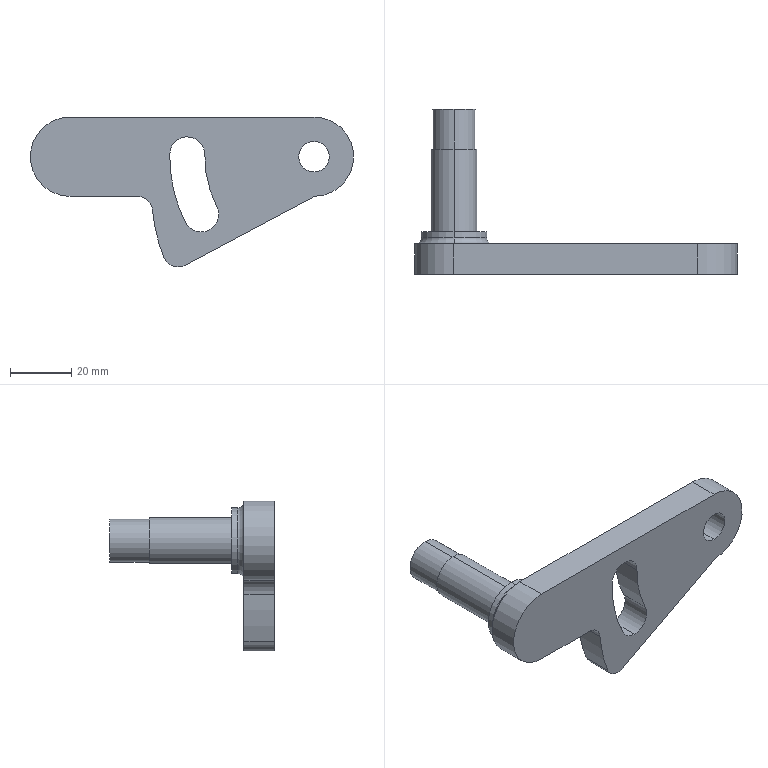Part | SolidWorks | features ICE 3, Fillet 2, Extrusion 1 | 1 solid | 30 faces | box 105.906 x 54 x 49.114 mm | volume 37118 mm3 | cylinder 20 | plane 8 | torus 2 | commonest cylinder face diameters 10 x5 11.5 x3 14 x2 15 x2 21.5 x2 26.001 x2
STEP:
#1=CARTESIAN_POINT('',(0.09446,54.,-6.));
#2=VERTEX_POINT('',#1);
#3=CARTESIAN_POINT('',(0.09446,54.,-20.));
#4=VERTEX_POINT('',#3);
#5=CARTESIAN_POINT('',(0.09446,54.,-13.));
#6=DIRECTION('',(0.,1.,0.));
#7=DIRECTION('',(0.,0.,1.));
#8=AXIS2_PLACEMENT_3D('',#5,#6,#7);
#9=CIRCLE('',#8,7.);
#10=EDGE_CURVE('',#2,#4,#9,.T.);
#11=ORIENTED_EDGE('',*,*,#10,.F.);
#12=CARTESIAN_POINT('',(0.09446,41.,-6.));
#13=VERTEX_POINT('',#12);
#14=CARTESIAN_POINT('',(0.09446,54.,-6.));
#15=DIRECTION('',(0.,-1.,0.));
#16=VECTOR('',#15,1000.);
#17=LINE('',#14,#16);
#18=EDGE_CURVE('',#2,#13,#17,.T.);
#19=ORIENTED_EDGE('',*,*,#18,.T.);
#20=CARTESIAN_POINT('',(0.09446,41.,-20.));
#21=VERTEX_POINT('',#20);
#22=CARTESIAN_POINT('',(0.09446,41.,-13.));
#23=DIRECTION('',(0.,1.,0.));
#24=DIRECTION('',(0.,0.,1.));
#25=AXIS2_PLACEMENT_3D('',#22,#23,#24);
#26=CIRCLE('',#25,7.);
#27=EDGE_CURVE('',#13,#21,#26,.T.);
#28=ORIENTED_EDGE('',*,*,#27,.T.);
#29=CARTESIAN_POINT('',(0.09446,54.,-20.));
#30=DIRECTION('',(0.,-1.,0.));
#31=VECTOR('',#30,1000.);
#32=LINE('',#29,#31);
#33=EDGE_CURVE('',#4,#21,#32,.T.);
#34=ORIENTED_EDGE('',*,*,#33,.F.);
#35=EDGE_LOOP('',(#11,#19,#28,#34));
#36=FACE_OUTER_BOUND('',#35,.T.);
#37=CARTESIAN_POINT('',(0.09446,54.,-13.));
#38=DIRECTION('',(0.,-1.,0.));
#39=DIRECTION('',(0.,0.,-1.));
#40=AXIS2_PLACEMENT_3D('',#37,#38,#39);
#41=CYLINDRICAL_SURFACE('',#40,7.);
#42=ADVANCED_FACE('',(#36),#41,.T.);
#43=CARTESIAN_POINT('',(0.09446,41.,-5.5));
#44=VERTEX_POINT('',#43);
#45=CARTESIAN_POINT('',(0.09446,41.,-20.5));
#46=VERTEX_POINT('',#45);
#47=CARTESIAN_POINT('',(0.09446,41.,-13.));
#48=DIRECTION('',(0.,1.,0.));
#49=DIRECTION('',(0.,0.,1.));
#50=AXIS2_PLACEMENT_3D('',#47,#48,#49);
#51=CIRCLE('',#50,7.5);
#52=EDGE_CURVE('',#44,#46,#51,.T.);
#53=ORIENTED_EDGE('',*,*,#52,.F.);
#54=CARTESIAN_POINT('',(0.09446,14.,-5.5));
#55=VERTEX_POINT('',#54);
#56=CARTESIAN_POINT('',(0.09446,41.,-5.5));
#57=DIRECTION('',(0.,-1.,0.));
#58=VECTOR('',#57,1000.);
#59=LINE('',#56,#58);
#60=EDGE_CURVE('',#44,#55,#59,.T.);
#61=ORIENTED_EDGE('',*,*,#60,.T.);
#62=CARTESIAN_POINT('',(0.09446,14.,-20.5));
#63=VERTEX_POINT('',#62);
#64=CARTESIAN_POINT('',(0.09446,14.,-13.));
#65=DIRECTION('',(0.,1.,0.));
#66=DIRECTION('',(0.,0.,1.));
#67=AXIS2_PLACEMENT_3D('',#64,#65,#66);
#68=CIRCLE('',#67,7.5);
#69=EDGE_CURVE('',#55,#63,#68,.T.);
#70=ORIENTED_EDGE('',*,*,#69,.T.);
#71=CARTESIAN_POINT('',(0.09446,41.,-20.5));
#72=DIRECTION('',(0.,-1.,0.));
#73=VECTOR('',#72,1000.);
#74=LINE('',#71,#73);
#75=EDGE_CURVE('',#46,#63,#74,.T.);
#76=ORIENTED_EDGE('',*,*,#75,.F.);
#77=EDGE_LOOP('',(#53,#61,#70,#76));
#78=FACE_OUTER_BOUND('',#77,.T.);
#79=CARTESIAN_POINT('',(0.09446,41.,-13.));
#80=DIRECTION('',(0.,-1.,0.));
#81=DIRECTION('',(0.,0.,-1.));
#82=AXIS2_PLACEMENT_3D('',#79,#80,#81);
#83=CYLINDRICAL_SURFACE('',#82,7.5);
#84=ADVANCED_FACE('',(#78),#83,.T.);
#85=CARTESIAN_POINT('',(0.09446,12.,-23.75));
#86=VERTEX_POINT('',#85);
#87=CARTESIAN_POINT('',(0.09446,12.,-2.25));
#88=VERTEX_POINT('',#87);
#89=CARTESIAN_POINT('',(0.09446,12.,-13.));
#90=DIRECTION('',(0.,1.,0.));
#91=DIRECTION('',(0.,0.,1.));
#92=AXIS2_PLACEMENT_3D('',#89,#90,#91);
#93=CIRCLE('',#92,10.75);
#94=EDGE_CURVE('',#86,#88,#93,.T.);
#95=ORIENTED_EDGE('',*,*,#94,.F.);
#96=CARTESIAN_POINT('',(0.09446,10.,-25.75));
#97=VERTEX_POINT('',#96);
#98=CARTESIAN_POINT('',(0.09446,12.,-25.75));
#99=DIRECTION('',(1.,0.,0.));
#100=DIRECTION('',(0.,0.,-1.));
#101=AXIS2_PLACEMENT_3D('',#98,#99,#100);
#102=CIRCLE('',#101,2.);
#103=EDGE_CURVE('',#86,#97,#102,.T.);
#104=ORIENTED_EDGE('',*,*,#103,.T.);
#105=CARTESIAN_POINT('',(0.09446,10.,-0.25));
#106=VERTEX_POINT('',#105);
#107=CARTESIAN_POINT('',(0.09446,10.,-13.));
#108=DIRECTION('',(0.,-1.,0.));
#109=DIRECTION('',(0.,0.,1.));
#110=AXIS2_PLACEMENT_3D('',#107,#108,#109);
#111=CIRCLE('',#110,12.75);
#112=EDGE_CURVE('',#106,#97,#111,.T.);
#113=ORIENTED_EDGE('',*,*,#112,.F.);
#114=CARTESIAN_POINT('',(0.09446,12.,-0.25));
#115=DIRECTION('',(-1.,0.,0.));
#116=DIRECTION('',(0.,0.,1.));
#117=AXIS2_PLACEMENT_3D('',#114,#115,#116);
#118=CIRCLE('',#117,2.);
#119=EDGE_CURVE('',#88,#106,#118,.T.);
#120=ORIENTED_EDGE('',*,*,#119,.F.);
#121=EDGE_LOOP('',(#95,#104,#113,#120));
#122=FACE_OUTER_BOUND('',#121,.T.);
#123=CARTESIAN_POINT('',(0.09446,12.,-13.));
#124=DIRECTION('',(0.,1.,0.));
#125=DIRECTION('',(0.,0.,1.));
#126=AXIS2_PLACEMENT_3D('',#123,#124,#125);
#127=TOROIDAL_SURFACE('',#126,12.75,2.);
#128=ADVANCED_FACE('',(#122),#127,.F.);
#129=CARTESIAN_POINT('',(0.09446,14.,-2.25));
#130=VERTEX_POINT('',#129);
#131=CARTESIAN_POINT('',(0.09446,14.,-23.75));
#132=VERTEX_POINT('',#131);
#133=CARTESIAN_POINT('',(0.09446,14.,-13.));
#134=DIRECTION('',(0.,1.,0.));
#135=DIRECTION('',(0.,0.,1.));
#136=AXIS2_PLACEMENT_3D('',#133,#134,#135);
#137=CIRCLE('',#136,10.75);
#138=EDGE_CURVE('',#130,#132,#137,.T.);
#139=ORIENTED_EDGE('',*,*,#138,.F.);
#140=CARTESIAN_POINT('',(0.09446,14.,-2.25));
#141=DIRECTION('',(0.,-1.,0.));
#142=VECTOR('',#141,1000.);
#143=LINE('',#140,#142);
#144=EDGE_CURVE('',#130,#88,#143,.T.);
#145=ORIENTED_EDGE('',*,*,#144,.T.);
#146=CARTESIAN_POINT('',(0.09446,12.,-13.));
#147=DIRECTION('',(0.,1.,0.));
#148=DIRECTION('',(0.,0.,1.));
#149=AXIS2_PLACEMENT_3D('',#146,#147,#148);
#150=CIRCLE('',#149,10.75);
#151=EDGE_CURVE('',#88,#86,#150,.T.);
#152=ORIENTED_EDGE('',*,*,#151,.T.);
#153=CARTESIAN_POINT('',(0.09446,14.,-23.75));
#154=DIRECTION('',(0.,-1.,0.));
#155=VECTOR('',#154,1000.);
#156=LINE('',#153,#155);
#157=EDGE_CURVE('',#132,#86,#156,.T.);
#158=ORIENTED_EDGE('',*,*,#157,.F.);
#159=EDGE_LOOP('',(#139,#145,#152,#158));
#160=FACE_OUTER_BOUND('',#159,.T.);
#161=CARTESIAN_POINT('',(0.09446,14.,-13.));
#162=DIRECTION('',(0.,-1.,0.));
#163=DIRECTION('',(0.,0.,-1.));
#164=AXIS2_PLACEMENT_3D('',#161,#162,#163);
#165=CYLINDRICAL_SURFACE('',#164,10.75);
#166=ADVANCED_FACE('',(#160),#165,.T.);
#167=CARTESIAN_POINT('',(35.469,10.,-49.114));
#168=VERTEX_POINT('',#167);
#169=CARTESIAN_POINT('',(30.834,10.,-45.991));
#170=VERTEX_POINT('',#169);
#171=CARTESIAN_POINT('',(35.469,10.,-44.114));
#172=DIRECTION('',(0.,1.,0.));
#173=DIRECTION('',(0.,0.,1.));
#174=AXIS2_PLACEMENT_3D('',#171,#172,#173);
#175=CIRCLE('',#174,5.);
#176=EDGE_CURVE('',#168,#170,#175,.T.);
#177=ORIENTED_EDGE('',*,*,#176,.F.);
#178=CARTESIAN_POINT('',(35.469,0.,-49.114));
#179=VERTEX_POINT('',#178);
#180=CARTESIAN_POINT('',(35.469,10.,-49.114));
#181=DIRECTION('',(0.,-1.,0.));
#182=VECTOR('',#181,1000.);
#183=LINE('',#180,#182);
#184=EDGE_CURVE('',#168,#179,#183,.T.);
#185=ORIENTED_EDGE('',*,*,#184,.T.);
#186=CARTESIAN_POINT('',(30.834,0.,-45.991));
#187=VERTEX_POINT('',#186);
#188=CARTESIAN_POINT('',(35.469,0.,-44.114));
#189=DIRECTION('',(0.,-1.,0.));
#190=DIRECTION('',(0.,0.,1.));
#191=AXIS2_PLACEMENT_3D('',#188,#189,#190);
#192=CIRCLE('',#191,5.);
#193=EDGE_CURVE('',#187,#179,#192,.T.);
#194=ORIENTED_EDGE('',*,*,#193,.F.);
#195=CARTESIAN_POINT('',(30.834,10.,-45.991));
#196=DIRECTION('',(0.,-1.,0.));
#197=VECTOR('',#196,1000.);
#198=LINE('',#195,#197);
#199=EDGE_CURVE('',#170,#187,#198,.T.);
#200=ORIENTED_EDGE('',*,*,#199,.F.);
#201=EDGE_LOOP('',(#177,#185,#194,#200));
#202=FACE_OUTER_BOUND('',#201,.T.);
#203=CARTESIAN_POINT('',(35.469,10.,-44.114));
#204=DIRECTION('',(0.,-1.,0.));
#205=DIRECTION('',(0.,0.,-1.));
#206=AXIS2_PLACEMENT_3D('',#203,#204,#205);
#207=CYLINDRICAL_SURFACE('',#206,5.);
#208=ADVANCED_FACE('',(#202),#207,.T.);
#209=CARTESIAN_POINT('',(48.162,10.,-29.261));
#210=VERTEX_POINT('',#209);
#211=CARTESIAN_POINT('',(43.041,10.,-37.626));
#212=VERTEX_POINT('',#211);
#213=CARTESIAN_POINT('',(43.041,10.,-31.876));
#214=DIRECTION('',(0.,1.,0.));
#215=DIRECTION('',(0.,0.,1.));
#216=AXIS2_PLACEMENT_3D('',#213,#214,#215);
#217=CIRCLE('',#216,5.75);
#218=EDGE_CURVE('',#210,#212,#217,.T.);
#219=ORIENTED_EDGE('',*,*,#218,.T.);
#220=CARTESIAN_POINT('',(43.041,0.,-37.626));
#221=VERTEX_POINT('',#220);
#222=CARTESIAN_POINT('',(43.041,10.,-37.626));
#223=DIRECTION('',(0.,-1.,0.));
#224=VECTOR('',#223,1000.);
#225=LINE('',#222,#224);
#226=EDGE_CURVE('',#212,#221,#225,.T.);
#227=ORIENTED_EDGE('',*,*,#226,.T.);
#228=CARTESIAN_POINT('',(48.162,0.,-29.261));
#229=VERTEX_POINT('',#228);
#230=CARTESIAN_POINT('',(43.041,0.,-31.876));
#231=DIRECTION('',(0.,1.,0.));
#232=DIRECTION('',(0.,0.,1.));
#233=AXIS2_PLACEMENT_3D('',#230,#231,#232);
#234=CIRCLE('',#233,5.75);
#235=EDGE_CURVE('',#229,#221,#234,.T.);
#236=ORIENTED_EDGE('',*,*,#235,.F.);
#237=CARTESIAN_POINT('',(48.162,10.,-29.261));
#238=DIRECTION('',(0.,-1.,0.));
#239=VECTOR('',#238,1000.);
#240=LINE('',#237,#239);
#241=EDGE_CURVE('',#210,#229,#240,.T.);
#242=ORIENTED_EDGE('',*,*,#241,.F.);
#243=EDGE_LOOP('',(#219,#227,#236,#242));
#244=FACE_OUTER_BOUND('',#243,.T.);
#245=CARTESIAN_POINT('',(43.041,10.,-31.876));
#246=DIRECTION('',(0.,-1.,0.));
#247=DIRECTION('',(0.,0.,-1.));
#248=AXIS2_PLACEMENT_3D('',#245,#246,#247);
#249=CYLINDRICAL_SURFACE('',#248,5.75);
#250=ADVANCED_FACE('',(#244),#249,.F.);
#251=CARTESIAN_POINT('',(80.,10.,-18.));
#252=VERTEX_POINT('',#251);
#253=CARTESIAN_POINT('',(80.,10.,-8.));
#254=VERTEX_POINT('',#253);
#255=CARTESIAN_POINT('',(80.,10.,-13.));
#256=DIRECTION('',(0.,1.,0.));
#257=DIRECTION('',(0.,0.,1.));
#258=AXIS2_PLACEMENT_3D('',#255,#256,#257);
#259=CIRCLE('',#258,5.);
#260=EDGE_CURVE('',#252,#254,#259,.T.);
#261=ORIENTED_EDGE('',*,*,#260,.T.);
#262=CARTESIAN_POINT('',(80.,0.,-8.));
#263=VERTEX_POINT('',#262);
#264=CARTESIAN_POINT('',(80.,10.,-8.));
#265=DIRECTION('',(0.,-1.,0.));
#266=VECTOR('',#265,1000.);
#267=LINE('',#264,#266);
#268=EDGE_CURVE('',#254,#263,#267,.T.);
#269=ORIENTED_EDGE('',*,*,#268,.T.);
#270=CARTESIAN_POINT('',(80.,0.,-18.));
#271=VERTEX_POINT('',#270);
#272=CARTESIAN_POINT('',(80.,0.,-13.));
#273=DIRECTION('',(0.,1.,0.));
#274=DIRECTION('',(0.,0.,1.));
#275=AXIS2_PLACEMENT_3D('',#272,#273,#274);
#276=CIRCLE('',#275,5.);
#277=EDGE_CURVE('',#271,#263,#276,.T.);
#278=ORIENTED_EDGE('',*,*,#277,.F.);
#279=CARTESIAN_POINT('',(80.,10.,-18.));
#280=DIRECTION('',(0.,-1.,0.));
#281=VECTOR('',#280,1000.);
#282=LINE('',#279,#281);
#283=EDGE_CURVE('',#252,#271,#282,.T.);
#284=ORIENTED_EDGE('',*,*,#283,.F.);
#285=EDGE_LOOP('',(#261,#269,#278,#284));
#286=FACE_OUTER_BOUND('',#285,.T.);
#287=CARTESIAN_POINT('',(80.,10.,-13.));
#288=DIRECTION('',(0.,-1.,0.));
#289=DIRECTION('',(0.,0.,-1.));
#290=AXIS2_PLACEMENT_3D('',#287,#288,#289);
#291=CYLINDRICAL_SURFACE('',#290,5.);
#292=ADVANCED_FACE('',(#286),#291,.F.);
#293=CARTESIAN_POINT('',(0.09446,10.,-26.));
#294=VERTEX_POINT('',#293);
#295=CARTESIAN_POINT('',(0.,10.,0.));
#296=VERTEX_POINT('',#295);
#297=CARTESIAN_POINT('',(0.09446,10.,-13.));
#298=DIRECTION('',(0.,1.,0.));
#299=DIRECTION('',(0.,0.,1.));
#300=AXIS2_PLACEMENT_3D('',#297,#298,#299);
#301=CIRCLE('',#300,13.);
#302=EDGE_CURVE('',#294,#296,#301,.T.);
#303=ORIENTED_EDGE('',*,*,#302,.F.);
#304=CARTESIAN_POINT('',(0.09446,0.,-26.));
#305=VERTEX_POINT('',#304);
#306=CARTESIAN_POINT('',(0.09446,10.,-26.));
#307=DIRECTION('',(0.,-1.,0.));
#308=VECTOR('',#307,1000.);
#309=LINE('',#306,#308);
#310=EDGE_CURVE('',#294,#305,#309,.T.);
#311=ORIENTED_EDGE('',*,*,#310,.T.);
#312=CARTESIAN_POINT('',(0.,0.,0.));
#313=VERTEX_POINT('',#312);
#314=CARTESIAN_POINT('',(0.09446,0.,-13.));
#315=DIRECTION('',(0.,1.,0.));
#316=DIRECTION('',(0.,0.,1.));
#317=AXIS2_PLACEMENT_3D('',#314,#315,#316);
#318=CIRCLE('',#317,13.);
#319=EDGE_CURVE('',#305,#313,#318,.T.);
#320=ORIENTED_EDGE('',*,*,#319,.T.);
#321=CARTESIAN_POINT('',(0.,10.,0.));
#322=DIRECTION('',(0.,-1.,0.));
#323=VECTOR('',#322,1000.);
#324=LINE('',#321,#323);
#325=EDGE_CURVE('',#296,#313,#324,.T.);
#326=ORIENTED_EDGE('',*,*,#325,.F.);
#327=EDGE_LOOP('',(#303,#311,#320,#326));
#328=FACE_OUTER_BOUND('',#327,.T.);
#329=CARTESIAN_POINT('',(0.09446,10.,-13.));
#330=DIRECTION('',(0.,-1.,0.));
#331=DIRECTION('',(0.,0.,-1.));
#332=AXIS2_PLACEMENT_3D('',#329,#330,#331);
#333=CYLINDRICAL_SURFACE('',#332,13.);
#334=ADVANCED_FACE('',(#328),#333,.T.);
#335=ORIENTED_EDGE('',*,*,#112,.T.);
#336=CARTESIAN_POINT('',(0.09446,10.,-13.));
#337=DIRECTION('',(0.,-1.,0.));
#338=DIRECTION('',(0.,0.,1.));
#339=AXIS2_PLACEMENT_3D('',#336,#337,#338);
#340=CIRCLE('',#339,12.75);
#341=EDGE_CURVE('',#97,#106,#340,.T.);
#342=ORIENTED_EDGE('',*,*,#341,.T.);
#343=EDGE_LOOP('',(#335,#342));
#344=FACE_BOUND('',#343,.T.);
#345=CARTESIAN_POINT('',(80.189,10.,-25.999));
#346=VERTEX_POINT('',#345);
#347=CARTESIAN_POINT('',(37.816,10.,-48.529));
#348=VERTEX_POINT('',#347);
#349=CARTESIAN_POINT('',(80.189,10.,-25.999));
#350=DIRECTION('',(-0.8829,0.,-0.4695));
#351=VECTOR('',#350,1000.);
#352=LINE('',#349,#351);
#353=EDGE_CURVE('',#346,#348,#352,.T.);
#354=ORIENTED_EDGE('',*,*,#353,.T.);
#355=CARTESIAN_POINT('',(35.469,10.,-44.114));
#356=DIRECTION('',(0.,1.,0.));
#357=DIRECTION('',(0.,0.,1.));
#358=AXIS2_PLACEMENT_3D('',#355,#356,#357);
#359=CIRCLE('',#358,5.);
#360=EDGE_CURVE('',#348,#168,#359,.T.);
#361=ORIENTED_EDGE('',*,*,#360,.T.);
#362=ORIENTED_EDGE('',*,*,#176,.T.);
#363=CARTESIAN_POINT('',(27.136,10.,-30.571));
#364=VERTEX_POINT('',#363);
#365=CARTESIAN_POINT('',(80.189,10.,-25.999));
#366=DIRECTION('',(0.,1.,0.));
#367=DIRECTION('',(0.,0.,1.));
#368=AXIS2_PLACEMENT_3D('',#365,#366,#367);
#369=CIRCLE('',#368,53.25);
#370=EDGE_CURVE('',#170,#364,#369,.T.);
#371=ORIENTED_EDGE('',*,*,#370,.T.);
#372=CARTESIAN_POINT('',(22.154,10.,-26.));
#373=VERTEX_POINT('',#372);
#374=CARTESIAN_POINT('',(22.154,10.,-31.));
#375=DIRECTION('',(0.,-1.,0.));
#376=DIRECTION('',(0.,0.,1.));
#377=AXIS2_PLACEMENT_3D('',#374,#375,#376);
#378=CIRCLE('',#377,5.);
#379=EDGE_CURVE('',#364,#373,#378,.T.);
#380=ORIENTED_EDGE('',*,*,#379,.T.);
#381=CARTESIAN_POINT('',(0.1889,10.,-26.));
#382=VERTEX_POINT('',#381);
#383=CARTESIAN_POINT('',(0.1889,10.,-26.));
#384=DIRECTION('',(-1.,0.,0.));
#385=VECTOR('',#384,1000.);
#386=LINE('',#383,#385);
#387=EDGE_CURVE('',#373,#382,#386,.T.);
#388=ORIENTED_EDGE('',*,*,#387,.T.);
#389=CARTESIAN_POINT('',(0.09446,10.,-13.));
#390=DIRECTION('',(0.,1.,0.));
#391=DIRECTION('',(0.,0.,1.));
#392=AXIS2_PLACEMENT_3D('',#389,#390,#391);
#393=CIRCLE('',#392,13.);
#394=EDGE_CURVE('',#382,#294,#393,.T.);
#395=ORIENTED_EDGE('',*,*,#394,.T.);
#396=ORIENTED_EDGE('',*,*,#302,.T.);
#397=CARTESIAN_POINT('',(80.,10.,0.));
#398=VERTEX_POINT('',#397);
#399=CARTESIAN_POINT('',(0.,10.,0.));
#400=DIRECTION('',(1.,0.,0.));
#401=VECTOR('',#400,1000.);
#402=LINE('',#399,#401);
#403=EDGE_CURVE('',#296,#398,#402,.T.);
#404=ORIENTED_EDGE('',*,*,#403,.T.);
#405=CARTESIAN_POINT('',(80.,10.,-13.));
#406=DIRECTION('',(0.,1.,0.));
#407=DIRECTION('',(0.,0.,1.));
#408=AXIS2_PLACEMENT_3D('',#405,#406,#407);
#409=CIRCLE('',#408,13.);
#410=EDGE_CURVE('',#398,#346,#409,.T.);
#411=ORIENTED_EDGE('',*,*,#410,.T.);
#412=EDGE_LOOP('',(#354,#361,#362,#371,#380,#388,#395,#396,#404,#411));
#413=FACE_OUTER_BOUND('',#412,.T.);
#414=ORIENTED_EDGE('',*,*,#260,.F.);
#415=CARTESIAN_POINT('',(80.,10.,-13.));
#416=DIRECTION('',(0.,1.,0.));
#417=DIRECTION('',(0.,0.,1.));
#418=AXIS2_PLACEMENT_3D('',#415,#416,#417);
#419=CIRCLE('',#418,5.);
#420=EDGE_CURVE('',#254,#252,#419,.T.);
#421=ORIENTED_EDGE('',*,*,#420,.F.);
#422=EDGE_LOOP('',(#414,#421));
#423=FACE_BOUND('',#422,.T.);
#424=CARTESIAN_POINT('',(37.921,10.,-34.492));
#425=VERTEX_POINT('',#424);
#426=CARTESIAN_POINT('',(32.758,10.,-12.146));
#427=VERTEX_POINT('',#426);
#428=CARTESIAN_POINT('',(80.,10.,-13.));
#429=DIRECTION('',(0.,1.,0.));
#430=DIRECTION('',(0.,0.,1.));
#431=AXIS2_PLACEMENT_3D('',#428,#429,#430);
#432=CIRCLE('',#431,47.25);
#433=EDGE_CURVE('',#425,#427,#432,.T.);
#434=ORIENTED_EDGE('',*,*,#433,.F.);
#435=CARTESIAN_POINT('',(43.041,10.,-31.876));
#436=DIRECTION('',(0.,1.,0.));
#437=DIRECTION('',(0.,0.,1.));
#438=AXIS2_PLACEMENT_3D('',#435,#436,#437);
#439=CIRCLE('',#438,5.75);
#440=EDGE_CURVE('',#212,#425,#439,.T.);
#441=ORIENTED_EDGE('',*,*,#440,.F.);
#442=ORIENTED_EDGE('',*,*,#218,.F.);
#443=CARTESIAN_POINT('',(44.256,10.,-12.354));
#444=VERTEX_POINT('',#443);
#445=CARTESIAN_POINT('',(80.,10.,-13.));
#446=DIRECTION('',(0.,-1.,0.));
#447=DIRECTION('',(0.,0.,1.));
#448=AXIS2_PLACEMENT_3D('',#445,#446,#447);
#449=CIRCLE('',#448,35.75);
#450=EDGE_CURVE('',#444,#210,#449,.T.);
#451=ORIENTED_EDGE('',*,*,#450,.F.);
#452=CARTESIAN_POINT('',(38.507,10.,-12.25));
#453=DIRECTION('',(0.,1.,0.));
#454=DIRECTION('',(0.,0.,1.));
#455=AXIS2_PLACEMENT_3D('',#452,#453,#454);
#456=CIRCLE('',#455,5.75);
#457=EDGE_CURVE('',#427,#444,#456,.T.);
#458=ORIENTED_EDGE('',*,*,#457,.F.);
#459=EDGE_LOOP('',(#434,#441,#442,#451,#458));
#460=FACE_BOUND('',#459,.T.);
#461=CARTESIAN_POINT('',(0.09446,10.,-13.));
#462=DIRECTION('',(0.,1.,0.));
#463=DIRECTION('',(0.,0.,1.));
#464=AXIS2_PLACEMENT_3D('',#461,#462,#463);
#465=PLANE('',#464);
#466=ADVANCED_FACE('',(#344,#413,#423,#460),#465,.T.);
#467=ORIENTED_EDGE('',*,*,#277,.T.);
#468=CARTESIAN_POINT('',(80.,0.,-13.));
#469=DIRECTION('',(0.,1.,0.));
#470=DIRECTION('',(0.,0.,1.));
#471=AXIS2_PLACEMENT_3D('',#468,#469,#470);
#472=CIRCLE('',#471,5.);
#473=EDGE_CURVE('',#263,#271,#472,.T.);
#474=ORIENTED_EDGE('',*,*,#473,.T.);
#475=EDGE_LOOP('',(#467,#474));
#476=FACE_BOUND('',#475,.T.);
#477=CARTESIAN_POINT('',(27.136,0.,-30.571));
#478=VERTEX_POINT('',#477);
#479=CARTESIAN_POINT('',(80.189,0.,-25.999));
#480=DIRECTION('',(0.,1.,0.));
#481=DIRECTION('',(0.,0.,1.));
#482=AXIS2_PLACEMENT_3D('',#479,#480,#481);
#483=CIRCLE('',#482,53.25);
#484=EDGE_CURVE('',#187,#478,#483,.T.);
#485=ORIENTED_EDGE('',*,*,#484,.F.);
#486=ORIENTED_EDGE('',*,*,#193,.T.);
#487=CARTESIAN_POINT('',(37.816,0.,-48.529));
#488=VERTEX_POINT('',#487);
#489=CARTESIAN_POINT('',(35.469,0.,-44.114));
#490=DIRECTION('',(0.,-1.,0.));
#491=DIRECTION('',(0.,0.,1.));
#492=AXIS2_PLACEMENT_3D('',#489,#490,#491);
#493=CIRCLE('',#492,5.);
#494=EDGE_CURVE('',#179,#488,#493,.T.);
#495=ORIENTED_EDGE('',*,*,#494,.T.);
#496=CARTESIAN_POINT('',(80.189,0.,-25.999));
#497=VERTEX_POINT('',#496);
#498=CARTESIAN_POINT('',(80.189,0.,-25.999));
#499=DIRECTION('',(-0.8829,0.,-0.4695));
#500=VECTOR('',#499,1000.);
#501=LINE('',#498,#500);
#502=EDGE_CURVE('',#497,#488,#501,.T.);
#503=ORIENTED_EDGE('',*,*,#502,.F.);
#504=CARTESIAN_POINT('',(80.,0.,0.));
#505=VERTEX_POINT('',#504);
#506=CARTESIAN_POINT('',(80.,0.,-13.));
#507=DIRECTION('',(0.,1.,0.));
#508=DIRECTION('',(0.,0.,1.));
#509=AXIS2_PLACEMENT_3D('',#506,#507,#508);
#510=CIRCLE('',#509,13.);
#511=EDGE_CURVE('',#505,#497,#510,.T.);
#512=ORIENTED_EDGE('',*,*,#511,.F.);
#513=CARTESIAN_POINT('',(0.,0.,0.));
#514=DIRECTION('',(1.,0.,0.));
#515=VECTOR('',#514,1000.);
#516=LINE('',#513,#515);
#517=EDGE_CURVE('',#313,#505,#516,.T.);
#518=ORIENTED_EDGE('',*,*,#517,.F.);
#519=ORIENTED_EDGE('',*,*,#319,.F.);
#520=CARTESIAN_POINT('',(0.1889,0.,-26.));
#521=VERTEX_POINT('',#520);
#522=CARTESIAN_POINT('',(0.09446,0.,-13.));
#523=DIRECTION('',(0.,1.,0.));
#524=DIRECTION('',(0.,0.,1.));
#525=AXIS2_PLACEMENT_3D('',#522,#523,#524);
#526=CIRCLE('',#525,13.);
#527=EDGE_CURVE('',#521,#305,#526,.T.);
#528=ORIENTED_EDGE('',*,*,#527,.F.);
#529=CARTESIAN_POINT('',(22.154,0.,-26.));
#530=VERTEX_POINT('',#529);
#531=CARTESIAN_POINT('',(0.1889,0.,-26.));
#532=DIRECTION('',(-1.,0.,0.));
#533=VECTOR('',#532,1000.);
#534=LINE('',#531,#533);
#535=EDGE_CURVE('',#530,#521,#534,.T.);
#536=ORIENTED_EDGE('',*,*,#535,.F.);
#537=CARTESIAN_POINT('',(22.154,0.,-31.));
#538=DIRECTION('',(0.,1.,0.));
#539=DIRECTION('',(0.,0.,1.));
#540=AXIS2_PLACEMENT_3D('',#537,#538,#539);
#541=CIRCLE('',#540,5.);
#542=EDGE_CURVE('',#530,#478,#541,.T.);
#543=ORIENTED_EDGE('',*,*,#542,.T.);
#544=EDGE_LOOP('',(#485,#486,#495,#503,#512,#518,#519,#528,#536,#543));
#545=FACE_OUTER_BOUND('',#544,.T.);
#546=ORIENTED_EDGE('',*,*,#235,.T.);
#547=CARTESIAN_POINT('',(37.921,0.,-34.492));
#548=VERTEX_POINT('',#547);
#549=CARTESIAN_POINT('',(43.041,0.,-31.876));
#550=DIRECTION('',(0.,1.,0.));
#551=DIRECTION('',(0.,0.,1.));
#552=AXIS2_PLACEMENT_3D('',#549,#550,#551);
#553=CIRCLE('',#552,5.75);
#554=EDGE_CURVE('',#221,#548,#553,.T.);
#555=ORIENTED_EDGE('',*,*,#554,.T.);
#556=CARTESIAN_POINT('',(32.758,0.,-12.146));
#557=VERTEX_POINT('',#556);
#558=CARTESIAN_POINT('',(80.,0.,-13.));
#559=DIRECTION('',(0.,1.,0.));
#560=DIRECTION('',(0.,0.,1.));
#561=AXIS2_PLACEMENT_3D('',#558,#559,#560);
#562=CIRCLE('',#561,47.25);
#563=EDGE_CURVE('',#548,#557,#562,.T.);
#564=ORIENTED_EDGE('',*,*,#563,.T.);
#565=CARTESIAN_POINT('',(44.256,0.,-12.354));
#566=VERTEX_POINT('',#565);
#567=CARTESIAN_POINT('',(38.507,0.,-12.25));
#568=DIRECTION('',(0.,1.,0.));
#569=DIRECTION('',(0.,0.,1.));
#570=AXIS2_PLACEMENT_3D('',#567,#568,#569);
#571=CIRCLE('',#570,5.75);
#572=EDGE_CURVE('',#557,#566,#571,.T.);
#573=ORIENTED_EDGE('',*,*,#572,.T.);
#574=CARTESIAN_POINT('',(80.,0.,-13.));
#575=DIRECTION('',(0.,-1.,0.));
#576=DIRECTION('',(0.,0.,1.));
#577=AXIS2_PLACEMENT_3D('',#574,#575,#576);
#578=CIRCLE('',#577,35.75);
#579=EDGE_CURVE('',#566,#229,#578,.T.);
#580=ORIENTED_EDGE('',*,*,#579,.T.);
#581=EDGE_LOOP('',(#546,#555,#564,#573,#580));
#582=FACE_BOUND('',#581,.T.);
#583=CARTESIAN_POINT('',(0.09446,0.,-13.));
#584=DIRECTION('',(0.,1.,0.));
#585=DIRECTION('',(0.,0.,1.));
#586=AXIS2_PLACEMENT_3D('',#583,#584,#585);
#587=PLANE('',#586);
#588=ADVANCED_FACE('',(#476,#545,#582),#587,.F.);
#589=ORIENTED_EDGE('',*,*,#310,.F.);
#590=ORIENTED_EDGE('',*,*,#394,.F.);
#591=CARTESIAN_POINT('',(0.1889,10.,-26.));
#592=DIRECTION('',(0.,-1.,0.));
#593=VECTOR('',#592,1000.);
#594=LINE('',#591,#593);
#595=EDGE_CURVE('',#382,#521,#594,.T.);
#596=ORIENTED_EDGE('',*,*,#595,.T.);
#597=ORIENTED_EDGE('',*,*,#527,.T.);
#598=EDGE_LOOP('',(#589,#590,#596,#597));
#599=FACE_OUTER_BOUND('',#598,.T.);
#600=CARTESIAN_POINT('',(0.09446,10.,-13.));
#601=DIRECTION('',(0.,-1.,0.));
#602=DIRECTION('',(0.,0.,-1.));
#603=AXIS2_PLACEMENT_3D('',#600,#601,#602);
#604=CYLINDRICAL_SURFACE('',#603,13.);
#605=ADVANCED_FACE('',(#599),#604,.T.);
#606=ORIENTED_EDGE('',*,*,#517,.T.);
#607=CARTESIAN_POINT('',(80.,10.,0.));
#608=DIRECTION('',(0.,-1.,0.));
#609=VECTOR('',#608,1000.);
#610=LINE('',#607,#609);
#611=EDGE_CURVE('',#398,#505,#610,.T.);
#612=ORIENTED_EDGE('',*,*,#611,.F.);
#613=ORIENTED_EDGE('',*,*,#403,.F.);
#614=ORIENTED_EDGE('',*,*,#325,.T.);
#615=EDGE_LOOP('',(#606,#612,#613,#614));
#616=FACE_OUTER_BOUND('',#615,.T.);
#617=CARTESIAN_POINT('',(0.,10.,0.));
#618=DIRECTION('',(0.,0.,-1.));
#619=DIRECTION('',(-1.,0.,0.));
#620=AXIS2_PLACEMENT_3D('',#617,#618,#619);
#621=PLANE('',#620);
#622=ADVANCED_FACE('',(#616),#621,.F.);
#623=ORIENTED_EDGE('',*,*,#511,.T.);
#624=CARTESIAN_POINT('',(80.189,10.,-25.999));
#625=DIRECTION('',(0.,-1.,0.));
#626=VECTOR('',#625,1000.);
#627=LINE('',#624,#626);
#628=EDGE_CURVE('',#346,#497,#627,.T.);
#629=ORIENTED_EDGE('',*,*,#628,.F.);
#630=ORIENTED_EDGE('',*,*,#410,.F.);
#631=ORIENTED_EDGE('',*,*,#611,.T.);
#632=EDGE_LOOP('',(#623,#629,#630,#631));
#633=FACE_OUTER_BOUND('',#632,.T.);
#634=CARTESIAN_POINT('',(80.,10.,-13.));
#635=DIRECTION('',(0.,-1.,0.));
#636=DIRECTION('',(0.,0.,-1.));
#637=AXIS2_PLACEMENT_3D('',#634,#635,#636);
#638=CYLINDRICAL_SURFACE('',#637,13.);
#639=ADVANCED_FACE('',(#633),#638,.T.);
#640=ORIENTED_EDGE('',*,*,#502,.T.);
#641=CARTESIAN_POINT('',(37.816,10.,-48.529));
#642=DIRECTION('',(0.,1.,0.));
#643=VECTOR('',#642,1000.);
#644=LINE('',#641,#643);
#645=EDGE_CURVE('',#488,#348,#644,.T.);
#646=ORIENTED_EDGE('',*,*,#645,.T.);
#647=ORIENTED_EDGE('',*,*,#353,.F.);
#648=ORIENTED_EDGE('',*,*,#628,.T.);
#649=EDGE_LOOP('',(#640,#646,#647,#648));
#650=FACE_OUTER_BOUND('',#649,.T.);
#651=CARTESIAN_POINT('',(80.189,10.,-25.999));
#652=DIRECTION('',(-0.4695,0.,0.8829));
#653=DIRECTION('',(0.8829,0.,0.4695));
#654=AXIS2_PLACEMENT_3D('',#651,#652,#653);
#655=PLANE('',#654);
#656=ADVANCED_FACE('',(#650),#655,.F.);
#657=ORIENTED_EDGE('',*,*,#484,.T.);
#658=CARTESIAN_POINT('',(27.136,10.,-30.571));
#659=DIRECTION('',(0.,1.,0.));
#660=VECTOR('',#659,1000.);
#661=LINE('',#658,#660);
#662=EDGE_CURVE('',#478,#364,#661,.T.);
#663=ORIENTED_EDGE('',*,*,#662,.T.);
#664=ORIENTED_EDGE('',*,*,#370,.F.);
#665=ORIENTED_EDGE('',*,*,#199,.T.);
#666=EDGE_LOOP('',(#657,#663,#664,#665));
#667=FACE_OUTER_BOUND('',#666,.T.);
#668=CARTESIAN_POINT('',(80.189,10.,-25.999));
#669=DIRECTION('',(0.,-1.,0.));
#670=DIRECTION('',(0.,0.,-1.));
#671=AXIS2_PLACEMENT_3D('',#668,#669,#670);
#672=CYLINDRICAL_SURFACE('',#671,53.25);
#673=ADVANCED_FACE('',(#667),#672,.T.);
#674=ORIENTED_EDGE('',*,*,#387,.F.);
#675=CARTESIAN_POINT('',(22.154,0.,-26.));
#676=DIRECTION('',(0.,-1.,0.));
#677=VECTOR('',#676,1000.);
#678=LINE('',#675,#677);
#679=EDGE_CURVE('',#373,#530,#678,.T.);
#680=ORIENTED_EDGE('',*,*,#679,.T.);
#681=ORIENTED_EDGE('',*,*,#535,.T.);
#682=ORIENTED_EDGE('',*,*,#595,.F.);
#683=EDGE_LOOP('',(#674,#680,#681,#682));
#684=FACE_OUTER_BOUND('',#683,.T.);
#685=CARTESIAN_POINT('',(0.1889,10.,-26.));
#686=DIRECTION('',(0.,0.,1.));
#687=DIRECTION('',(1.,0.,0.));
#688=AXIS2_PLACEMENT_3D('',#685,#686,#687);
#689=PLANE('',#688);
#690=ADVANCED_FACE('',(#684),#689,.F.);
#691=ORIENTED_EDGE('',*,*,#268,.F.);
#692=ORIENTED_EDGE('',*,*,#420,.T.);
#693=ORIENTED_EDGE('',*,*,#283,.T.);
#694=ORIENTED_EDGE('',*,*,#473,.F.);
#695=EDGE_LOOP('',(#691,#692,#693,#694));
#696=FACE_OUTER_BOUND('',#695,.T.);
#697=CARTESIAN_POINT('',(80.,10.,-13.));
#698=DIRECTION('',(0.,-1.,0.));
#699=DIRECTION('',(0.,0.,-1.));
#700=AXIS2_PLACEMENT_3D('',#697,#698,#699);
#701=CYLINDRICAL_SURFACE('',#700,5.);
#702=ADVANCED_FACE('',(#696),#701,.F.);
#703=ORIENTED_EDGE('',*,*,#226,.F.);
#704=ORIENTED_EDGE('',*,*,#440,.T.);
#705=CARTESIAN_POINT('',(37.921,10.,-34.492));
#706=DIRECTION('',(0.,-1.,0.));
#707=VECTOR('',#706,1000.);
#708=LINE('',#705,#707);
#709=EDGE_CURVE('',#425,#548,#708,.T.);
#710=ORIENTED_EDGE('',*,*,#709,.T.);
#711=ORIENTED_EDGE('',*,*,#554,.F.);
#712=EDGE_LOOP('',(#703,#704,#710,#711));
#713=FACE_OUTER_BOUND('',#712,.T.);
#714=CARTESIAN_POINT('',(43.041,10.,-31.876));
#715=DIRECTION('',(0.,-1.,0.));
#716=DIRECTION('',(0.,0.,-1.));
#717=AXIS2_PLACEMENT_3D('',#714,#715,#716);
#718=CYLINDRICAL_SURFACE('',#717,5.75);
#719=ADVANCED_FACE('',(#713),#718,.F.);
#720=ORIENTED_EDGE('',*,*,#563,.F.);
#721=ORIENTED_EDGE('',*,*,#709,.F.);
#722=ORIENTED_EDGE('',*,*,#433,.T.);
#723=CARTESIAN_POINT('',(32.758,10.,-12.146));
#724=DIRECTION('',(0.,-1.,0.));
#725=VECTOR('',#724,1000.);
#726=LINE('',#723,#725);
#727=EDGE_CURVE('',#427,#557,#726,.T.);
#728=ORIENTED_EDGE('',*,*,#727,.T.);
#729=EDGE_LOOP('',(#720,#721,#722,#728));
#730=FACE_OUTER_BOUND('',#729,.T.);
#731=CARTESIAN_POINT('',(80.,10.,-13.));
#732=DIRECTION('',(0.,-1.,0.));
#733=DIRECTION('',(0.,0.,-1.));
#734=AXIS2_PLACEMENT_3D('',#731,#732,#733);
#735=CYLINDRICAL_SURFACE('',#734,47.25);
#736=ADVANCED_FACE('',(#730),#735,.F.);
#737=ORIENTED_EDGE('',*,*,#572,.F.);
#738=ORIENTED_EDGE('',*,*,#727,.F.);
#739=ORIENTED_EDGE('',*,*,#457,.T.);
#740=CARTESIAN_POINT('',(44.256,10.,-12.354));
#741=DIRECTION('',(0.,-1.,0.));
#742=VECTOR('',#741,1000.);
#743=LINE('',#740,#742);
#744=EDGE_CURVE('',#444,#566,#743,.T.);
#745=ORIENTED_EDGE('',*,*,#744,.T.);
#746=EDGE_LOOP('',(#737,#738,#739,#745));
#747=FACE_OUTER_BOUND('',#746,.T.);
#748=CARTESIAN_POINT('',(38.507,10.,-12.25));
#749=DIRECTION('',(0.,-1.,0.));
#750=DIRECTION('',(0.,0.,-1.));
#751=AXIS2_PLACEMENT_3D('',#748,#749,#750);
#752=CYLINDRICAL_SURFACE('',#751,5.75);
#753=ADVANCED_FACE('',(#747),#752,.F.);
#754=ORIENTED_EDGE('',*,*,#579,.F.);
#755=ORIENTED_EDGE('',*,*,#744,.F.);
#756=ORIENTED_EDGE('',*,*,#450,.T.);
#757=ORIENTED_EDGE('',*,*,#241,.T.);
#758=EDGE_LOOP('',(#754,#755,#756,#757));
#759=FACE_OUTER_BOUND('',#758,.T.);
#760=CARTESIAN_POINT('',(80.,10.,-13.));
#761=DIRECTION('',(0.,-1.,0.));
#762=DIRECTION('',(0.,0.,-1.));
#763=AXIS2_PLACEMENT_3D('',#760,#761,#762);
#764=CYLINDRICAL_SURFACE('',#763,35.75);
#765=ADVANCED_FACE('',(#759),#764,.T.);
#766=ORIENTED_EDGE('',*,*,#379,.F.);
#767=ORIENTED_EDGE('',*,*,#662,.F.);
#768=ORIENTED_EDGE('',*,*,#542,.F.);
#769=ORIENTED_EDGE('',*,*,#679,.F.);
#770=EDGE_LOOP('',(#766,#767,#768,#769));
#771=FACE_OUTER_BOUND('',#770,.T.);
#772=CARTESIAN_POINT('',(22.154,10.,-31.));
#773=DIRECTION('',(0.,-1.,0.));
#774=DIRECTION('',(0.,0.,-1.));
#775=AXIS2_PLACEMENT_3D('',#772,#773,#774);
#776=CYLINDRICAL_SURFACE('',#775,5.);
#777=ADVANCED_FACE('',(#771),#776,.F.);
#778=ORIENTED_EDGE('',*,*,#184,.F.);
#779=ORIENTED_EDGE('',*,*,#360,.F.);
#780=ORIENTED_EDGE('',*,*,#645,.F.);
#781=ORIENTED_EDGE('',*,*,#494,.F.);
#782=EDGE_LOOP('',(#778,#779,#780,#781));
#783=FACE_OUTER_BOUND('',#782,.T.);
#784=CARTESIAN_POINT('',(35.469,10.,-44.114));
#785=DIRECTION('',(0.,-1.,0.));
#786=DIRECTION('',(0.,0.,-1.));
#787=AXIS2_PLACEMENT_3D('',#784,#785,#786);
#788=CYLINDRICAL_SURFACE('',#787,5.);
#789=ADVANCED_FACE('',(#783),#788,.T.);
#790=ORIENTED_EDGE('',*,*,#144,.F.);
#791=CARTESIAN_POINT('',(0.09446,14.,-13.));
#792=DIRECTION('',(0.,1.,0.));
#793=DIRECTION('',(0.,0.,1.));
#794=AXIS2_PLACEMENT_3D('',#791,#792,#793);
#795=CIRCLE('',#794,10.75);
#796=EDGE_CURVE('',#132,#130,#795,.T.);
#797=ORIENTED_EDGE('',*,*,#796,.F.);
#798=ORIENTED_EDGE('',*,*,#157,.T.);
#799=ORIENTED_EDGE('',*,*,#94,.T.);
#800=EDGE_LOOP('',(#790,#797,#798,#799));
#801=FACE_OUTER_BOUND('',#800,.T.);
#802=CARTESIAN_POINT('',(0.09446,14.,-13.));
#803=DIRECTION('',(0.,-1.,0.));
#804=DIRECTION('',(0.,0.,-1.));
#805=AXIS2_PLACEMENT_3D('',#802,#803,#804);
#806=CYLINDRICAL_SURFACE('',#805,10.75);
#807=ADVANCED_FACE('',(#801),#806,.T.);
#808=CARTESIAN_POINT('',(0.09446,14.,-13.));
#809=DIRECTION('',(0.,1.,0.));
#810=DIRECTION('',(0.,0.,1.));
#811=AXIS2_PLACEMENT_3D('',#808,#809,#810);
#812=CIRCLE('',#811,7.5);
#813=EDGE_CURVE('',#63,#55,#812,.T.);
#814=ORIENTED_EDGE('',*,*,#813,.F.);
#815=ORIENTED_EDGE('',*,*,#69,.F.);
#816=EDGE_LOOP('',(#814,#815));
#817=FACE_BOUND('',#816,.T.);
#818=ORIENTED_EDGE('',*,*,#796,.T.);
#819=ORIENTED_EDGE('',*,*,#138,.T.);
#820=EDGE_LOOP('',(#818,#819));
#821=FACE_OUTER_BOUND('',#820,.T.);
#822=CARTESIAN_POINT('',(0.09446,14.,-13.));
#823=DIRECTION('',(0.,1.,0.));
#824=DIRECTION('',(0.,0.,1.));
#825=AXIS2_PLACEMENT_3D('',#822,#823,#824);
#826=PLANE('',#825);
#827=ADVANCED_FACE('',(#817,#821),#826,.T.);
#828=ORIENTED_EDGE('',*,*,#103,.F.);
#829=ORIENTED_EDGE('',*,*,#151,.F.);
#830=ORIENTED_EDGE('',*,*,#119,.T.);
#831=ORIENTED_EDGE('',*,*,#341,.F.);
#832=EDGE_LOOP('',(#828,#829,#830,#831));
#833=FACE_OUTER_BOUND('',#832,.T.);
#834=CARTESIAN_POINT('',(0.09446,12.,-13.));
#835=DIRECTION('',(0.,1.,0.));
#836=DIRECTION('',(0.,0.,1.));
#837=AXIS2_PLACEMENT_3D('',#834,#835,#836);
#838=TOROIDAL_SURFACE('',#837,12.75,2.);
#839=ADVANCED_FACE('',(#833),#838,.F.);
#840=ORIENTED_EDGE('',*,*,#60,.F.);
#841=CARTESIAN_POINT('',(0.09446,41.,-13.));
#842=DIRECTION('',(0.,1.,0.));
#843=DIRECTION('',(0.,0.,1.));
#844=AXIS2_PLACEMENT_3D('',#841,#842,#843);
#845=CIRCLE('',#844,7.5);
#846=EDGE_CURVE('',#46,#44,#845,.T.);
#847=ORIENTED_EDGE('',*,*,#846,.F.);
#848=ORIENTED_EDGE('',*,*,#75,.T.);
#849=ORIENTED_EDGE('',*,*,#813,.T.);
#850=EDGE_LOOP('',(#840,#847,#848,#849));
#851=FACE_OUTER_BOUND('',#850,.T.);
#852=CARTESIAN_POINT('',(0.09446,41.,-13.));
#853=DIRECTION('',(0.,-1.,0.));
#854=DIRECTION('',(0.,0.,-1.));
#855=AXIS2_PLACEMENT_3D('',#852,#853,#854);
#856=CYLINDRICAL_SURFACE('',#855,7.5);
#857=ADVANCED_FACE('',(#851),#856,.T.);
#858=CARTESIAN_POINT('',(0.09446,41.,-13.));
#859=DIRECTION('',(0.,1.,0.));
#860=DIRECTION('',(0.,0.,1.));
#861=AXIS2_PLACEMENT_3D('',#858,#859,#860);
#862=CIRCLE('',#861,7.);
#863=EDGE_CURVE('',#21,#13,#862,.T.);
#864=ORIENTED_EDGE('',*,*,#863,.F.);
#865=ORIENTED_EDGE('',*,*,#27,.F.);
#866=EDGE_LOOP('',(#864,#865));
#867=FACE_BOUND('',#866,.T.);
#868=ORIENTED_EDGE('',*,*,#846,.T.);
#869=ORIENTED_EDGE('',*,*,#52,.T.);
#870=EDGE_LOOP('',(#868,#869));
#871=FACE_OUTER_BOUND('',#870,.T.);
#872=CARTESIAN_POINT('',(0.09446,41.,-13.));
#873=DIRECTION('',(0.,1.,0.));
#874=DIRECTION('',(0.,0.,1.));
#875=AXIS2_PLACEMENT_3D('',#872,#873,#874);
#876=PLANE('',#875);
#877=ADVANCED_FACE('',(#867,#871),#876,.T.);
#878=ORIENTED_EDGE('',*,*,#18,.F.);
#879=CARTESIAN_POINT('',(0.09446,54.,-13.));
#880=DIRECTION('',(0.,1.,0.));
#881=DIRECTION('',(0.,0.,1.));
#882=AXIS2_PLACEMENT_3D('',#879,#880,#881);
#883=CIRCLE('',#882,7.);
#884=EDGE_CURVE('',#4,#2,#883,.T.);
#885=ORIENTED_EDGE('',*,*,#884,.F.);
#886=ORIENTED_EDGE('',*,*,#33,.T.);
#887=ORIENTED_EDGE('',*,*,#863,.T.);
#888=EDGE_LOOP('',(#878,#885,#886,#887));
#889=FACE_OUTER_BOUND('',#888,.T.);
#890=CARTESIAN_POINT('',(0.09446,54.,-13.));
#891=DIRECTION('',(0.,-1.,0.));
#892=DIRECTION('',(0.,0.,-1.));
#893=AXIS2_PLACEMENT_3D('',#890,#891,#892);
#894=CYLINDRICAL_SURFACE('',#893,7.);
#895=ADVANCED_FACE('',(#889),#894,.T.);
#896=ORIENTED_EDGE('',*,*,#884,.T.);
#897=ORIENTED_EDGE('',*,*,#10,.T.);
#898=EDGE_LOOP('',(#896,#897));
#899=FACE_OUTER_BOUND('',#898,.T.);
#900=CARTESIAN_POINT('',(0.09446,54.,-13.));
#901=DIRECTION('',(0.,1.,0.));
#902=DIRECTION('',(0.,0.,1.));
#903=AXIS2_PLACEMENT_3D('',#900,#901,#902);
#904=PLANE('',#903);
#905=ADVANCED_FACE('',(#899),#904,.T.);
#906=CLOSED_SHELL('',(#42,#84,#128,#166,#208,#250,#292,#334,#466,#588,#605,#622,#639,#656,#673,#690,#702,#719,#736,#753,#765,#777,#789,#807,#827,#839,#857,#877,#895,#905));
#907=MANIFOLD_SOLID_BREP('',#906);
#908=CARTESIAN_POINT('',(0.,0.,0.));
#909=DIRECTION('',(0.,0.,1.));
#910=DIRECTION('',(1.,0.,0.));
#911=AXIS2_PLACEMENT_3D('',#908,#909,#910);
#912=(LENGTH_UNIT()NAMED_UNIT(*)SI_UNIT(.MILLI.,.METRE.));
#913=UNCERTAINTY_MEASURE_WITH_UNIT(LENGTH_MEASURE(0.00001),#912,'','');
#914=(NAMED_UNIT(*)PLANE_ANGLE_UNIT()SI_UNIT($,.RADIAN.));
#915=(NAMED_UNIT(*)SI_UNIT($,.STERADIAN.)SOLID_ANGLE_UNIT());
#916=(GEOMETRIC_REPRESENTATION_CONTEXT(3)GLOBAL_UNCERTAINTY_ASSIGNED_CONTEXT((#913))GLOBAL_UNIT_ASSIGNED_CONTEXT((#912,#914,#915))REPRESENTATION_CONTEXT('',''));
#917=ADVANCED_BREP_SHAPE_REPRESENTATION('',(#907,#911),#916);